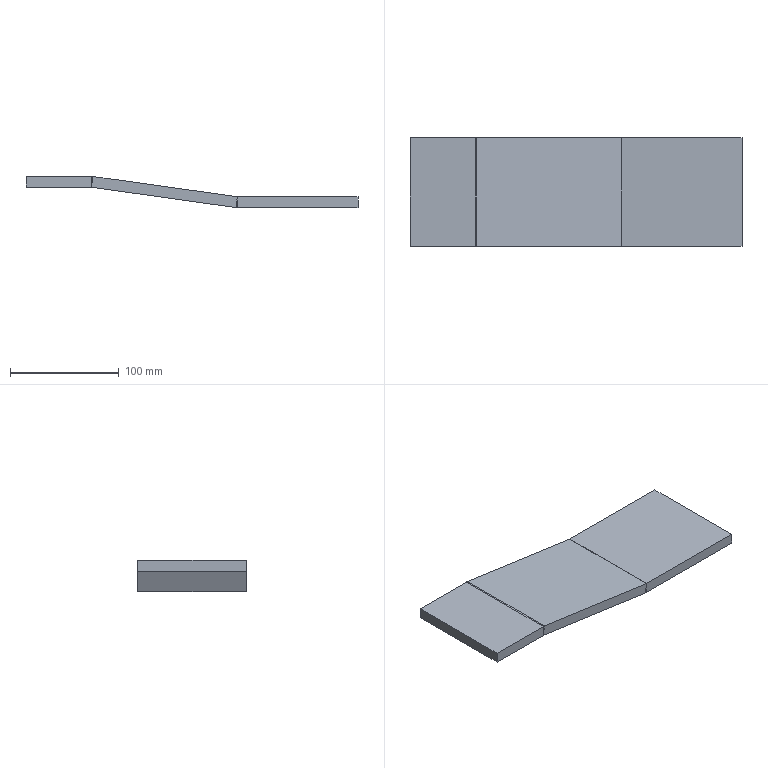Part | STEP file | C1 | 1 solid | 22 faces | box 305.395 x 100 x 28.803 mm | volume 306707 mm3 | plane 18 | cylinder 4 | commonest cylinder face diameters 3 x2 23 x2
STEP:
#1=CARTESIAN_POINT('',(0.,0.,0.));
#2=DIRECTION('',(0.,0.,1.));
#3=DIRECTION('',(1.,0.,0.));
#4=AXIS2_PLACEMENT_3D('',#1,#2,#3);
#5=CARTESIAN_POINT('',(0.,100.,0.));
#6=VERTEX_POINT('',#5);
#7=CARTESIAN_POINT('',(0.,0.,0.));
#8=VERTEX_POINT('',#7);
#9=CARTESIAN_POINT('',(0.,100.,0.));
#10=DIRECTION('',(0.,-1.,0.));
#11=VECTOR('',#10,1.);
#12=LINE('',#9,#11);
#13=CARTESIAN_POINT('',(0.,100.,-10.));
#14=DIRECTION('',(-1.,0.,0.));
#15=DIRECTION('',(0.,-1.,0.));
#16=AXIS2_PLACEMENT_3D('',#13,#14,#15);
#17=PLANE('',#16);
#18=CARTESIAN_POINT('',(0.,10.));
#19=DIRECTION('',(1.,0.));
#20=VECTOR('',#19,1.);
#21=LINE('',#18,#20);
#22=(GEOMETRIC_REPRESENTATION_CONTEXT(2)PARAMETRIC_REPRESENTATION_CONTEXT()REPRESENTATION_CONTEXT('',''));
#23=DEFINITIONAL_REPRESENTATION('',(#21),#22);
#24=PCURVE('',#17,#23);
#25=CARTESIAN_POINT('',(0.,0.,0.));
#26=DIRECTION('',(0.,0.,1.));
#27=DIRECTION('',(1.,0.,0.));
#28=AXIS2_PLACEMENT_3D('',#25,#26,#27);
#29=PLANE('',#28);
#30=CARTESIAN_POINT('',(0.,100.));
#31=DIRECTION('',(0.,-1.));
#32=VECTOR('',#31,1.);
#33=LINE('',#30,#32);
#34=(GEOMETRIC_REPRESENTATION_CONTEXT(2)PARAMETRIC_REPRESENTATION_CONTEXT()REPRESENTATION_CONTEXT('',''));
#35=DEFINITIONAL_REPRESENTATION('',(#33),#34);
#36=PCURVE('',#29,#35);
#37=SURFACE_CURVE('',#12,(#24,#36),.PCURVE_S1.);
#38=EDGE_CURVE('',#6,#8,#37,.T.);
#39=ORIENTED_EDGE('',*,*,#38,.F.);
#40=CARTESIAN_POINT('',(0.,100.,-10.));
#41=VERTEX_POINT('',#40);
#42=CARTESIAN_POINT('',(0.,100.,-10.));
#43=DIRECTION('',(0.,0.,1.));
#44=VECTOR('',#43,1.);
#45=LINE('',#42,#44);
#46=CARTESIAN_POINT('',(0.,0.));
#47=DIRECTION('',(0.,1.));
#48=VECTOR('',#47,1.);
#49=LINE('',#46,#48);
#50=(GEOMETRIC_REPRESENTATION_CONTEXT(2)PARAMETRIC_REPRESENTATION_CONTEXT()REPRESENTATION_CONTEXT('',''));
#51=DEFINITIONAL_REPRESENTATION('',(#49),#50);
#52=PCURVE('',#17,#51);
#53=CARTESIAN_POINT('',(0.,100.,-10.));
#54=DIRECTION('',(0.,1.,0.));
#55=DIRECTION('',(-1.,0.,0.));
#56=AXIS2_PLACEMENT_3D('',#53,#54,#55);
#57=PLANE('',#56);
#58=CARTESIAN_POINT('',(0.,0.));
#59=DIRECTION('',(0.,1.));
#60=VECTOR('',#59,1.);
#61=LINE('',#58,#60);
#62=(GEOMETRIC_REPRESENTATION_CONTEXT(2)PARAMETRIC_REPRESENTATION_CONTEXT()REPRESENTATION_CONTEXT('',''));
#63=DEFINITIONAL_REPRESENTATION('',(#61),#62);
#64=PCURVE('',#57,#63);
#65=SURFACE_CURVE('',#45,(#52,#64),.PCURVE_S1.);
#66=EDGE_CURVE('',#41,#6,#65,.T.);
#67=ORIENTED_EDGE('',*,*,#66,.F.);
#68=CARTESIAN_POINT('',(0.,0.,-10.));
#69=VERTEX_POINT('',#68);
#70=CARTESIAN_POINT('',(0.,100.,-10.));
#71=DIRECTION('',(0.,-1.,0.));
#72=VECTOR('',#71,1.);
#73=LINE('',#70,#72);
#74=CARTESIAN_POINT('',(0.,0.));
#75=DIRECTION('',(1.,0.));
#76=VECTOR('',#75,1.);
#77=LINE('',#74,#76);
#78=(GEOMETRIC_REPRESENTATION_CONTEXT(2)PARAMETRIC_REPRESENTATION_CONTEXT()REPRESENTATION_CONTEXT('',''));
#79=DEFINITIONAL_REPRESENTATION('',(#77),#78);
#80=PCURVE('',#17,#79);
#81=CARTESIAN_POINT('',(0.,0.,-10.));
#82=DIRECTION('',(0.,0.,1.));
#83=DIRECTION('',(1.,0.,0.));
#84=AXIS2_PLACEMENT_3D('',#81,#82,#83);
#85=PLANE('',#84);
#86=CARTESIAN_POINT('',(0.,100.));
#87=DIRECTION('',(0.,-1.));
#88=VECTOR('',#87,1.);
#89=LINE('',#86,#88);
#90=(GEOMETRIC_REPRESENTATION_CONTEXT(2)PARAMETRIC_REPRESENTATION_CONTEXT()REPRESENTATION_CONTEXT('',''));
#91=DEFINITIONAL_REPRESENTATION('',(#89),#90);
#92=PCURVE('',#85,#91);
#93=SURFACE_CURVE('',#73,(#80,#92),.PCURVE_S1.);
#94=EDGE_CURVE('',#41,#69,#93,.T.);
#95=ORIENTED_EDGE('',*,*,#94,.T.);
#96=CARTESIAN_POINT('',(0.,0.,-10.));
#97=DIRECTION('',(0.,0.,1.));
#98=VECTOR('',#97,1.);
#99=LINE('',#96,#98);
#100=CARTESIAN_POINT('',(100.,0.));
#101=DIRECTION('',(0.,1.));
#102=VECTOR('',#101,1.);
#103=LINE('',#100,#102);
#104=(GEOMETRIC_REPRESENTATION_CONTEXT(2)PARAMETRIC_REPRESENTATION_CONTEXT()REPRESENTATION_CONTEXT('',''));
#105=DEFINITIONAL_REPRESENTATION('',(#103),#104);
#106=PCURVE('',#17,#105);
#107=CARTESIAN_POINT('',(0.,0.,-10.));
#108=DIRECTION('',(0.,-1.,0.));
#109=DIRECTION('',(1.,0.,0.));
#110=AXIS2_PLACEMENT_3D('',#107,#108,#109);
#111=PLANE('',#110);
#112=CARTESIAN_POINT('',(0.,0.));
#113=DIRECTION('',(0.,1.));
#114=VECTOR('',#113,1.);
#115=LINE('',#112,#114);
#116=(GEOMETRIC_REPRESENTATION_CONTEXT(2)PARAMETRIC_REPRESENTATION_CONTEXT()REPRESENTATION_CONTEXT('',''));
#117=DEFINITIONAL_REPRESENTATION('',(#115),#116);
#118=PCURVE('',#111,#117);
#119=SURFACE_CURVE('',#99,(#106,#118),.PCURVE_S1.);
#120=EDGE_CURVE('',#69,#8,#119,.T.);
#121=ORIENTED_EDGE('',*,*,#120,.T.);
#122=EDGE_LOOP('',(#39,#67,#95,#121));
#123=FACE_BOUND('',#122,.T.);
#124=ADVANCED_FACE('',(#123),#17,.T.);
#125=CARTESIAN_POINT('',(60.,100.,0.));
#126=VERTEX_POINT('',#125);
#127=CARTESIAN_POINT('',(0.,100.,0.));
#128=DIRECTION('',(-1.,0.,0.));
#129=VECTOR('',#128,1.);
#130=LINE('',#127,#129);
#131=CARTESIAN_POINT('',(0.,10.));
#132=DIRECTION('',(1.,0.));
#133=VECTOR('',#132,1.);
#134=LINE('',#131,#133);
#135=(GEOMETRIC_REPRESENTATION_CONTEXT(2)PARAMETRIC_REPRESENTATION_CONTEXT()REPRESENTATION_CONTEXT('',''));
#136=DEFINITIONAL_REPRESENTATION('',(#134),#135);
#137=PCURVE('',#57,#136);
#138=CARTESIAN_POINT('',(0.,100.));
#139=DIRECTION('',(-1.,0.));
#140=VECTOR('',#139,1.);
#141=LINE('',#138,#140);
#142=(GEOMETRIC_REPRESENTATION_CONTEXT(2)PARAMETRIC_REPRESENTATION_CONTEXT()REPRESENTATION_CONTEXT('',''));
#143=DEFINITIONAL_REPRESENTATION('',(#141),#142);
#144=PCURVE('',#29,#143);
#145=SURFACE_CURVE('',#130,(#137,#144),.PCURVE_S1.);
#146=EDGE_CURVE('',#126,#6,#145,.T.);
#147=ORIENTED_EDGE('',*,*,#146,.F.);
#148=CARTESIAN_POINT('',(60.,100.,-10.));
#149=VERTEX_POINT('',#148);
#150=CARTESIAN_POINT('',(60.,100.,-10.));
#151=DIRECTION('',(0.,0.,1.));
#152=VECTOR('',#151,1.);
#153=LINE('',#150,#152);
#154=CARTESIAN_POINT('',(-60.,0.));
#155=DIRECTION('',(0.,1.));
#156=VECTOR('',#155,1.);
#157=LINE('',#154,#156);
#158=(GEOMETRIC_REPRESENTATION_CONTEXT(2)PARAMETRIC_REPRESENTATION_CONTEXT()REPRESENTATION_CONTEXT('',''));
#159=DEFINITIONAL_REPRESENTATION('',(#157),#158);
#160=PCURVE('',#57,#159);
#161=CARTESIAN_POINT('',(60.,100.,-11.5));
#162=DIRECTION('',(0.,1.,0.));
#163=DIRECTION('',(0.,0.,1.));
#164=AXIS2_PLACEMENT_3D('',#161,#162,#163);
#165=PLANE('',#164);
#166=CARTESIAN_POINT('',(1.5,0.));
#167=DIRECTION('',(1.,0.));
#168=VECTOR('',#167,1.);
#169=LINE('',#166,#168);
#170=(GEOMETRIC_REPRESENTATION_CONTEXT(2)PARAMETRIC_REPRESENTATION_CONTEXT()REPRESENTATION_CONTEXT('',''));
#171=DEFINITIONAL_REPRESENTATION('',(#169),#170);
#172=PCURVE('',#165,#171);
#173=SURFACE_CURVE('',#153,(#160,#172),.PCURVE_S1.);
#174=EDGE_CURVE('',#149,#126,#173,.T.);
#175=ORIENTED_EDGE('',*,*,#174,.F.);
#176=CARTESIAN_POINT('',(0.,100.,-10.));
#177=DIRECTION('',(-1.,0.,0.));
#178=VECTOR('',#177,1.);
#179=LINE('',#176,#178);
#180=CARTESIAN_POINT('',(0.,0.));
#181=DIRECTION('',(1.,0.));
#182=VECTOR('',#181,1.);
#183=LINE('',#180,#182);
#184=(GEOMETRIC_REPRESENTATION_CONTEXT(2)PARAMETRIC_REPRESENTATION_CONTEXT()REPRESENTATION_CONTEXT('',''));
#185=DEFINITIONAL_REPRESENTATION('',(#183),#184);
#186=PCURVE('',#57,#185);
#187=CARTESIAN_POINT('',(0.,100.));
#188=DIRECTION('',(-1.,0.));
#189=VECTOR('',#188,1.);
#190=LINE('',#187,#189);
#191=(GEOMETRIC_REPRESENTATION_CONTEXT(2)PARAMETRIC_REPRESENTATION_CONTEXT()REPRESENTATION_CONTEXT('',''));
#192=DEFINITIONAL_REPRESENTATION('',(#190),#191);
#193=PCURVE('',#85,#192);
#194=SURFACE_CURVE('',#179,(#186,#193),.PCURVE_S1.);
#195=EDGE_CURVE('',#149,#41,#194,.T.);
#196=ORIENTED_EDGE('',*,*,#195,.T.);
#197=ORIENTED_EDGE('',*,*,#66,.T.);
#198=EDGE_LOOP('',(#147,#175,#196,#197));
#199=FACE_BOUND('',#198,.T.);
#200=ADVANCED_FACE('',(#199),#57,.T.);
#201=CARTESIAN_POINT('',(60.,0.,0.));
#202=VERTEX_POINT('',#201);
#203=CARTESIAN_POINT('',(0.,0.,0.));
#204=DIRECTION('',(1.,0.,0.));
#205=VECTOR('',#204,1.);
#206=LINE('',#203,#205);
#207=CARTESIAN_POINT('',(0.,10.));
#208=DIRECTION('',(1.,0.));
#209=VECTOR('',#208,1.);
#210=LINE('',#207,#209);
#211=(GEOMETRIC_REPRESENTATION_CONTEXT(2)PARAMETRIC_REPRESENTATION_CONTEXT()REPRESENTATION_CONTEXT('',''));
#212=DEFINITIONAL_REPRESENTATION('',(#210),#211);
#213=PCURVE('',#111,#212);
#214=CARTESIAN_POINT('',(0.,0.));
#215=DIRECTION('',(1.,0.));
#216=VECTOR('',#215,1.);
#217=LINE('',#214,#216);
#218=(GEOMETRIC_REPRESENTATION_CONTEXT(2)PARAMETRIC_REPRESENTATION_CONTEXT()REPRESENTATION_CONTEXT('',''));
#219=DEFINITIONAL_REPRESENTATION('',(#217),#218);
#220=PCURVE('',#29,#219);
#221=SURFACE_CURVE('',#206,(#213,#220),.PCURVE_S1.);
#222=EDGE_CURVE('',#8,#202,#221,.T.);
#223=ORIENTED_EDGE('',*,*,#222,.F.);
#224=ORIENTED_EDGE('',*,*,#120,.F.);
#225=CARTESIAN_POINT('',(60.,0.,-10.));
#226=VERTEX_POINT('',#225);
#227=CARTESIAN_POINT('',(0.,0.,-10.));
#228=DIRECTION('',(1.,0.,0.));
#229=VECTOR('',#228,1.);
#230=LINE('',#227,#229);
#231=CARTESIAN_POINT('',(0.,0.));
#232=DIRECTION('',(1.,0.));
#233=VECTOR('',#232,1.);
#234=LINE('',#231,#233);
#235=(GEOMETRIC_REPRESENTATION_CONTEXT(2)PARAMETRIC_REPRESENTATION_CONTEXT()REPRESENTATION_CONTEXT('',''));
#236=DEFINITIONAL_REPRESENTATION('',(#234),#235);
#237=PCURVE('',#111,#236);
#238=CARTESIAN_POINT('',(0.,0.));
#239=DIRECTION('',(1.,0.));
#240=VECTOR('',#239,1.);
#241=LINE('',#238,#240);
#242=(GEOMETRIC_REPRESENTATION_CONTEXT(2)PARAMETRIC_REPRESENTATION_CONTEXT()REPRESENTATION_CONTEXT('',''));
#243=DEFINITIONAL_REPRESENTATION('',(#241),#242);
#244=PCURVE('',#85,#243);
#245=SURFACE_CURVE('',#230,(#237,#244),.PCURVE_S1.);
#246=EDGE_CURVE('',#69,#226,#245,.T.);
#247=ORIENTED_EDGE('',*,*,#246,.T.);
#248=CARTESIAN_POINT('',(60.,0.,-10.));
#249=DIRECTION('',(0.,0.,1.));
#250=VECTOR('',#249,1.);
#251=LINE('',#248,#250);
#252=CARTESIAN_POINT('',(60.,0.));
#253=DIRECTION('',(0.,1.));
#254=VECTOR('',#253,1.);
#255=LINE('',#252,#254);
#256=(GEOMETRIC_REPRESENTATION_CONTEXT(2)PARAMETRIC_REPRESENTATION_CONTEXT()REPRESENTATION_CONTEXT('',''));
#257=DEFINITIONAL_REPRESENTATION('',(#255),#256);
#258=PCURVE('',#111,#257);
#259=CARTESIAN_POINT('',(60.,0.,-11.5));
#260=DIRECTION('',(0.,1.,0.));
#261=DIRECTION('',(0.,0.,1.));
#262=AXIS2_PLACEMENT_3D('',#259,#260,#261);
#263=PLANE('',#262);
#264=CARTESIAN_POINT('',(1.5,0.));
#265=DIRECTION('',(1.,0.));
#266=VECTOR('',#265,1.);
#267=LINE('',#264,#266);
#268=(GEOMETRIC_REPRESENTATION_CONTEXT(2)PARAMETRIC_REPRESENTATION_CONTEXT()REPRESENTATION_CONTEXT('',''));
#269=DEFINITIONAL_REPRESENTATION('',(#267),#268);
#270=PCURVE('',#263,#269);
#271=SURFACE_CURVE('',#251,(#258,#270),.PCURVE_S1.);
#272=EDGE_CURVE('',#226,#202,#271,.T.);
#273=ORIENTED_EDGE('',*,*,#272,.T.);
#274=EDGE_LOOP('',(#223,#224,#247,#273));
#275=FACE_BOUND('',#274,.T.);
#276=ADVANCED_FACE('',(#275),#111,.T.);
#277=ORIENTED_EDGE('',*,*,#94,.F.);
#278=ORIENTED_EDGE('',*,*,#195,.F.);
#279=CARTESIAN_POINT('',(60.,100.,-10.));
#280=DIRECTION('',(0.,1.,0.));
#281=VECTOR('',#280,1.);
#282=LINE('',#279,#281);
#283=CARTESIAN_POINT('',(60.,100.));
#284=DIRECTION('',(0.,1.));
#285=VECTOR('',#284,1.);
#286=LINE('',#283,#285);
#287=(GEOMETRIC_REPRESENTATION_CONTEXT(2)PARAMETRIC_REPRESENTATION_CONTEXT()REPRESENTATION_CONTEXT('',''));
#288=DEFINITIONAL_REPRESENTATION('',(#286),#287);
#289=PCURVE('',#85,#288);
#290=CARTESIAN_POINT('',(60.,0.,-11.5));
#291=DIRECTION('',(0.,-1.,0.));
#292=DIRECTION('',(0.1392,0.,0.9903));
#293=AXIS2_PLACEMENT_3D('',#290,#291,#292);
#294=CYLINDRICAL_SURFACE('',#293,1.5);
#295=CARTESIAN_POINT('',(0.1396,-100.));
#296=DIRECTION('',(0.,-1.));
#297=VECTOR('',#296,1.);
#298=LINE('',#295,#297);
#299=(GEOMETRIC_REPRESENTATION_CONTEXT(2)PARAMETRIC_REPRESENTATION_CONTEXT()REPRESENTATION_CONTEXT('',''));
#300=DEFINITIONAL_REPRESENTATION('',(#298),#299);
#301=PCURVE('',#294,#300);
#302=SURFACE_CURVE('',#282,(#289,#301),.PCURVE_S1.);
#303=EDGE_CURVE('',#226,#149,#302,.T.);
#304=ORIENTED_EDGE('',*,*,#303,.F.);
#305=ORIENTED_EDGE('',*,*,#246,.F.);
#306=EDGE_LOOP('',(#277,#278,#304,#305));
#307=FACE_BOUND('',#306,.T.);
#308=ADVANCED_FACE('',(#307),#85,.F.);
#309=ORIENTED_EDGE('',*,*,#38,.T.);
#310=ORIENTED_EDGE('',*,*,#222,.T.);
#311=CARTESIAN_POINT('',(60.,100.,0.));
#312=DIRECTION('',(0.,1.,0.));
#313=VECTOR('',#312,1.);
#314=LINE('',#311,#313);
#315=CARTESIAN_POINT('',(60.,100.));
#316=DIRECTION('',(0.,1.));
#317=VECTOR('',#316,1.);
#318=LINE('',#315,#317);
#319=(GEOMETRIC_REPRESENTATION_CONTEXT(2)PARAMETRIC_REPRESENTATION_CONTEXT()REPRESENTATION_CONTEXT('',''));
#320=DEFINITIONAL_REPRESENTATION('',(#318),#319);
#321=PCURVE('',#29,#320);
#322=CARTESIAN_POINT('',(60.,0.,-11.5));
#323=DIRECTION('',(0.,-1.,0.));
#324=DIRECTION('',(0.1392,0.,0.9903));
#325=AXIS2_PLACEMENT_3D('',#322,#323,#324);
#326=CYLINDRICAL_SURFACE('',#325,11.5);
#327=CARTESIAN_POINT('',(0.1396,-100.));
#328=DIRECTION('',(0.,-1.));
#329=VECTOR('',#328,1.);
#330=LINE('',#327,#329);
#331=(GEOMETRIC_REPRESENTATION_CONTEXT(2)PARAMETRIC_REPRESENTATION_CONTEXT()REPRESENTATION_CONTEXT('',''));
#332=DEFINITIONAL_REPRESENTATION('',(#330),#331);
#333=PCURVE('',#326,#332);
#334=SURFACE_CURVE('',#314,(#321,#333),.PCURVE_S1.);
#335=EDGE_CURVE('',#202,#126,#334,.T.);
#336=ORIENTED_EDGE('',*,*,#335,.T.);
#337=ORIENTED_EDGE('',*,*,#146,.T.);
#338=EDGE_LOOP('',(#309,#310,#336,#337));
#339=FACE_BOUND('',#338,.T.);
#340=ADVANCED_FACE('',(#339),#29,.T.);
#341=CARTESIAN_POINT('',(60.209,100.,-10.015));
#342=VERTEX_POINT('',#341);
#343=CARTESIAN_POINT('',(61.6,100.,-0.1119));
#344=VERTEX_POINT('',#343);
#345=CARTESIAN_POINT('',(61.6,100.,-0.1119));
#346=DIRECTION('',(0.1392,0.,0.9903));
#347=VECTOR('',#346,1.);
#348=LINE('',#345,#347);
#349=CARTESIAN_POINT('',(11.388,1.6));
#350=DIRECTION('',(0.9903,0.1392));
#351=VECTOR('',#350,1.);
#352=LINE('',#349,#351);
#353=(GEOMETRIC_REPRESENTATION_CONTEXT(2)PARAMETRIC_REPRESENTATION_CONTEXT()REPRESENTATION_CONTEXT('',''));
#354=DEFINITIONAL_REPRESENTATION('',(#352),#353);
#355=PCURVE('',#165,#354);
#356=CARTESIAN_POINT('',(194.49,100.,-18.788));
#357=DIRECTION('',(0.,1.,0.));
#358=DIRECTION('',(-1.,0.,0.));
#359=AXIS2_PLACEMENT_3D('',#356,#357,#358);
#360=PLANE('',#359);
#361=CARTESIAN_POINT('',(132.89,18.676));
#362=DIRECTION('',(-0.1392,0.9903));
#363=VECTOR('',#362,1.);
#364=LINE('',#361,#363);
#365=(GEOMETRIC_REPRESENTATION_CONTEXT(2)PARAMETRIC_REPRESENTATION_CONTEXT()REPRESENTATION_CONTEXT('',''));
#366=DEFINITIONAL_REPRESENTATION('',(#364),#365);
#367=PCURVE('',#360,#366);
#368=SURFACE_CURVE('',#348,(#355,#367),.PCURVE_S1.);
#369=EDGE_CURVE('',#342,#344,#368,.T.);
#370=ORIENTED_EDGE('',*,*,#369,.F.);
#371=CARTESIAN_POINT('',(60.,100.,-11.5));
#372=DIRECTION('',(0.,1.,0.));
#373=DIRECTION('',(0.,0.,-1.));
#374=AXIS2_PLACEMENT_3D('',#371,#372,#373);
#375=CIRCLE('',#374,1.5);
#376=CARTESIAN_POINT('',(0.,0.));
#377=DIRECTION('',(-1.,0.));
#378=AXIS2_PLACEMENT_2D('',#376,#377);
#379=CIRCLE('',#378,1.5);
#380=(GEOMETRIC_REPRESENTATION_CONTEXT(2)PARAMETRIC_REPRESENTATION_CONTEXT()REPRESENTATION_CONTEXT('',''));
#381=DEFINITIONAL_REPRESENTATION('',(#379),#380);
#382=PCURVE('',#165,#381);
#383=CARTESIAN_POINT('',(3.281,-100.));
#384=DIRECTION('',(-1.,0.));
#385=VECTOR('',#384,1.);
#386=LINE('',#383,#385);
#387=(GEOMETRIC_REPRESENTATION_CONTEXT(2)PARAMETRIC_REPRESENTATION_CONTEXT()REPRESENTATION_CONTEXT('',''));
#388=DEFINITIONAL_REPRESENTATION('',(#386),#387);
#389=PCURVE('',#294,#388);
#390=SURFACE_CURVE('',#375,(#382,#389),.PCURVE_S1.);
#391=EDGE_CURVE('',#149,#342,#390,.T.);
#392=ORIENTED_EDGE('',*,*,#391,.F.);
#393=ORIENTED_EDGE('',*,*,#174,.T.);
#394=CARTESIAN_POINT('',(60.,100.,-11.5));
#395=DIRECTION('',(0.,1.,0.));
#396=DIRECTION('',(0.,0.,-1.));
#397=AXIS2_PLACEMENT_3D('',#394,#395,#396);
#398=CIRCLE('',#397,11.5);
#399=CARTESIAN_POINT('',(0.,0.));
#400=DIRECTION('',(-1.,0.));
#401=AXIS2_PLACEMENT_2D('',#399,#400);
#402=CIRCLE('',#401,11.5);
#403=(GEOMETRIC_REPRESENTATION_CONTEXT(2)PARAMETRIC_REPRESENTATION_CONTEXT()REPRESENTATION_CONTEXT('',''));
#404=DEFINITIONAL_REPRESENTATION('',(#402),#403);
#405=PCURVE('',#165,#404);
#406=CARTESIAN_POINT('',(3.281,-100.));
#407=DIRECTION('',(-1.,0.));
#408=VECTOR('',#407,1.);
#409=LINE('',#406,#408);
#410=(GEOMETRIC_REPRESENTATION_CONTEXT(2)PARAMETRIC_REPRESENTATION_CONTEXT()REPRESENTATION_CONTEXT('',''));
#411=DEFINITIONAL_REPRESENTATION('',(#409),#410);
#412=PCURVE('',#326,#411);
#413=SURFACE_CURVE('',#398,(#405,#412),.PCURVE_S1.);
#414=EDGE_CURVE('',#126,#344,#413,.T.);
#415=ORIENTED_EDGE('',*,*,#414,.T.);
#416=EDGE_LOOP('',(#370,#392,#393,#415));
#417=FACE_BOUND('',#416,.T.);
#418=ADVANCED_FACE('',(#417),#165,.T.);
#419=CARTESIAN_POINT('',(60.209,0.,-10.015));
#420=VERTEX_POINT('',#419);
#421=CARTESIAN_POINT('',(60.,0.,-11.5));
#422=DIRECTION('',(0.,-1.,0.));
#423=DIRECTION('',(0.,0.,-1.));
#424=AXIS2_PLACEMENT_3D('',#421,#422,#423);
#425=CIRCLE('',#424,1.5);
#426=CARTESIAN_POINT('',(-1.5,0.));
#427=CARTESIAN_POINT('',(-1.5,2.598));
#428=CARTESIAN_POINT('',(0.75,1.299));
#429=CARTESIAN_POINT('',(3.,0.));
#430=CARTESIAN_POINT('',(0.75,-1.299));
#431=CARTESIAN_POINT('',(-1.5,-2.598));
#432=CARTESIAN_POINT('',(-1.5,0.));
#433=(BOUNDED_CURVE()B_SPLINE_CURVE(2,(#426,#427,#428,#429,#430,#431,#432),.UNSPECIFIED.,.T.,.F.)B_SPLINE_CURVE_WITH_KNOTS((1,2,2,2,2,1),(-2.094,0.,2.094,4.189,6.283,8.378),.UNSPECIFIED.)CURVE()GEOMETRIC_REPRESENTATION_ITEM()RATIONAL_B_SPLINE_CURVE((1.,0.5,1.,0.5,1.,0.5,1.))REPRESENTATION_ITEM(''));
#434=(GEOMETRIC_REPRESENTATION_CONTEXT(2)PARAMETRIC_REPRESENTATION_CONTEXT()REPRESENTATION_CONTEXT('',''));
#435=DEFINITIONAL_REPRESENTATION('',(#433),#434);
#436=PCURVE('',#263,#435);
#437=CARTESIAN_POINT('',(-3.002,0.));
#438=DIRECTION('',(1.,0.));
#439=VECTOR('',#438,1.);
#440=LINE('',#437,#439);
#441=(GEOMETRIC_REPRESENTATION_CONTEXT(2)PARAMETRIC_REPRESENTATION_CONTEXT()REPRESENTATION_CONTEXT('',''));
#442=DEFINITIONAL_REPRESENTATION('',(#440),#441);
#443=PCURVE('',#294,#442);
#444=SURFACE_CURVE('',#425,(#436,#443),.PCURVE_S1.);
#445=EDGE_CURVE('',#420,#226,#444,.T.);
#446=ORIENTED_EDGE('',*,*,#445,.F.);
#447=CARTESIAN_POINT('',(61.6,0.,-0.1119));
#448=VERTEX_POINT('',#447);
#449=CARTESIAN_POINT('',(60.209,0.,-10.015));
#450=DIRECTION('',(0.1392,0.,0.9903));
#451=VECTOR('',#450,1.);
#452=LINE('',#449,#451);
#453=CARTESIAN_POINT('',(1.485,0.2088));
#454=DIRECTION('',(0.9903,0.1392));
#455=VECTOR('',#454,1.);
#456=LINE('',#453,#455);
#457=(GEOMETRIC_REPRESENTATION_CONTEXT(2)PARAMETRIC_REPRESENTATION_CONTEXT()REPRESENTATION_CONTEXT('',''));
#458=DEFINITIONAL_REPRESENTATION('',(#456),#457);
#459=PCURVE('',#263,#458);
#460=CARTESIAN_POINT('',(61.497,0.,-0.09732));
#461=DIRECTION('',(0.,-1.,0.));
#462=DIRECTION('',(1.,0.,0.));
#463=AXIS2_PLACEMENT_3D('',#460,#461,#462);
#464=PLANE('',#463);
#465=CARTESIAN_POINT('',(-1.288,-9.917));
#466=DIRECTION('',(0.1392,0.9903));
#467=VECTOR('',#466,1.);
#468=LINE('',#465,#467);
#469=(GEOMETRIC_REPRESENTATION_CONTEXT(2)PARAMETRIC_REPRESENTATION_CONTEXT()REPRESENTATION_CONTEXT('',''));
#470=DEFINITIONAL_REPRESENTATION('',(#468),#469);
#471=PCURVE('',#464,#470);
#472=SURFACE_CURVE('',#452,(#459,#471),.PCURVE_S1.);
#473=EDGE_CURVE('',#420,#448,#472,.T.);
#474=ORIENTED_EDGE('',*,*,#473,.T.);
#475=CARTESIAN_POINT('',(60.,0.,-11.5));
#476=DIRECTION('',(0.,-1.,0.));
#477=DIRECTION('',(0.,0.,-1.));
#478=AXIS2_PLACEMENT_3D('',#475,#476,#477);
#479=CIRCLE('',#478,11.5);
#480=CARTESIAN_POINT('',(-11.5,0.));
#481=CARTESIAN_POINT('',(-11.5,19.919));
#482=CARTESIAN_POINT('',(5.75,9.959));
#483=CARTESIAN_POINT('',(23.,0.));
#484=CARTESIAN_POINT('',(5.75,-9.959));
#485=CARTESIAN_POINT('',(-11.5,-19.919));
#486=CARTESIAN_POINT('',(-11.5,0.));
#487=(BOUNDED_CURVE()B_SPLINE_CURVE(2,(#480,#481,#482,#483,#484,#485,#486),.UNSPECIFIED.,.T.,.F.)B_SPLINE_CURVE_WITH_KNOTS((1,2,2,2,2,1),(-2.094,0.,2.094,4.189,6.283,8.378),.UNSPECIFIED.)CURVE()GEOMETRIC_REPRESENTATION_ITEM()RATIONAL_B_SPLINE_CURVE((1.,0.5,1.,0.5,1.,0.5,1.))REPRESENTATION_ITEM(''));
#488=(GEOMETRIC_REPRESENTATION_CONTEXT(2)PARAMETRIC_REPRESENTATION_CONTEXT()REPRESENTATION_CONTEXT('',''));
#489=DEFINITIONAL_REPRESENTATION('',(#487),#488);
#490=PCURVE('',#263,#489);
#491=CARTESIAN_POINT('',(-3.002,0.));
#492=DIRECTION('',(1.,0.));
#493=VECTOR('',#492,1.);
#494=LINE('',#491,#493);
#495=(GEOMETRIC_REPRESENTATION_CONTEXT(2)PARAMETRIC_REPRESENTATION_CONTEXT()REPRESENTATION_CONTEXT('',''));
#496=DEFINITIONAL_REPRESENTATION('',(#494),#495);
#497=PCURVE('',#326,#496);
#498=SURFACE_CURVE('',#479,(#490,#497),.PCURVE_S1.);
#499=EDGE_CURVE('',#448,#202,#498,.T.);
#500=ORIENTED_EDGE('',*,*,#499,.T.);
#501=ORIENTED_EDGE('',*,*,#272,.F.);
#502=EDGE_LOOP('',(#446,#474,#500,#501));
#503=FACE_BOUND('',#502,.T.);
#504=ADVANCED_FACE('',(#503),#263,.F.);
#505=ORIENTED_EDGE('',*,*,#335,.F.);
#506=ORIENTED_EDGE('',*,*,#499,.F.);
#507=CARTESIAN_POINT('',(61.6,0.,-0.1119));
#508=DIRECTION('',(0.,-1.,0.));
#509=VECTOR('',#508,1.);
#510=LINE('',#507,#509);
#511=CARTESIAN_POINT('',(0.,0.));
#512=DIRECTION('',(0.,1.));
#513=VECTOR('',#512,1.);
#514=LINE('',#511,#513);
#515=(GEOMETRIC_REPRESENTATION_CONTEXT(2)PARAMETRIC_REPRESENTATION_CONTEXT()REPRESENTATION_CONTEXT('',''));
#516=DEFINITIONAL_REPRESENTATION('',(#514),#515);
#517=PCURVE('',#326,#516);
#518=CARTESIAN_POINT('',(1.281,0.,8.365));
#519=DIRECTION('',(0.1392,0.,0.9903));
#520=DIRECTION('',(0.9903,0.,-0.1392));
#521=AXIS2_PLACEMENT_3D('',#518,#519,#520);
#522=PLANE('',#521);
#523=CARTESIAN_POINT('',(60.913,0.));
#524=DIRECTION('',(0.,-1.));
#525=VECTOR('',#524,1.);
#526=LINE('',#523,#525);
#527=(GEOMETRIC_REPRESENTATION_CONTEXT(2)PARAMETRIC_REPRESENTATION_CONTEXT()REPRESENTATION_CONTEXT('',''));
#528=DEFINITIONAL_REPRESENTATION('',(#526),#527);
#529=PCURVE('',#522,#528);
#530=SURFACE_CURVE('',#510,(#517,#529),.PCURVE_S1.);
#531=EDGE_CURVE('',#344,#448,#530,.T.);
#532=ORIENTED_EDGE('',*,*,#531,.F.);
#533=ORIENTED_EDGE('',*,*,#414,.F.);
#534=EDGE_LOOP('',(#505,#506,#532,#533));
#535=FACE_BOUND('',#534,.T.);
#536=ADVANCED_FACE('',(#535),#326,.T.);
#537=ORIENTED_EDGE('',*,*,#445,.F.);
#538=CARTESIAN_POINT('',(60.209,100.,-10.015));
#539=DIRECTION('',(0.,-1.,0.));
#540=VECTOR('',#539,1.);
#541=LINE('',#538,#540);
#542=CARTESIAN_POINT('',(0.,-100.));
#543=DIRECTION('',(0.,1.));
#544=VECTOR('',#543,1.);
#545=LINE('',#542,#544);
#546=(GEOMETRIC_REPRESENTATION_CONTEXT(2)PARAMETRIC_REPRESENTATION_CONTEXT()REPRESENTATION_CONTEXT('',''));
#547=DEFINITIONAL_REPRESENTATION('',(#545),#546);
#548=PCURVE('',#294,#547);
#549=CARTESIAN_POINT('',(-0.1111,0.,-1.537));
#550=DIRECTION('',(0.1392,0.,0.9903));
#551=DIRECTION('',(0.9903,0.,-0.1392));
#552=AXIS2_PLACEMENT_3D('',#549,#550,#551);
#553=PLANE('',#552);
#554=CARTESIAN_POINT('',(60.913,100.));
#555=DIRECTION('',(0.,-1.));
#556=VECTOR('',#555,1.);
#557=LINE('',#554,#556);
#558=(GEOMETRIC_REPRESENTATION_CONTEXT(2)PARAMETRIC_REPRESENTATION_CONTEXT()REPRESENTATION_CONTEXT('',''));
#559=DEFINITIONAL_REPRESENTATION('',(#557),#558);
#560=PCURVE('',#553,#559);
#561=SURFACE_CURVE('',#541,(#548,#560),.PCURVE_S1.);
#562=EDGE_CURVE('',#342,#420,#561,.T.);
#563=ORIENTED_EDGE('',*,*,#562,.F.);
#564=ORIENTED_EDGE('',*,*,#391,.F.);
#565=ORIENTED_EDGE('',*,*,#303,.F.);
#566=EDGE_LOOP('',(#537,#563,#564,#565));
#567=FACE_BOUND('',#566,.F.);
#568=ADVANCED_FACE('',(#567),#294,.F.);
#569=CARTESIAN_POINT('',(194.49,0.,-18.788));
#570=VERTEX_POINT('',#569);
#571=CARTESIAN_POINT('',(61.497,0.,-0.09732));
#572=DIRECTION('',(-0.9903,0.,0.1392));
#573=VECTOR('',#572,1.);
#574=LINE('',#571,#573);
#575=CARTESIAN_POINT('',(0.,0.));
#576=DIRECTION('',(-0.9903,0.1392));
#577=VECTOR('',#576,1.);
#578=LINE('',#575,#577);
#579=(GEOMETRIC_REPRESENTATION_CONTEXT(2)PARAMETRIC_REPRESENTATION_CONTEXT()REPRESENTATION_CONTEXT('',''));
#580=DEFINITIONAL_REPRESENTATION('',(#578),#579);
#581=PCURVE('',#464,#580);
#582=CARTESIAN_POINT('',(60.808,0.));
#583=DIRECTION('',(-1.,0.));
#584=VECTOR('',#583,1.);
#585=LINE('',#582,#584);
#586=(GEOMETRIC_REPRESENTATION_CONTEXT(2)PARAMETRIC_REPRESENTATION_CONTEXT()REPRESENTATION_CONTEXT('',''));
#587=DEFINITIONAL_REPRESENTATION('',(#585),#586);
#588=PCURVE('',#522,#587);
#589=SURFACE_CURVE('',#574,(#581,#588),.PCURVE_S1.);
#590=EDGE_CURVE('',#570,#448,#589,.T.);
#591=ORIENTED_EDGE('',*,*,#590,.T.);
#592=ORIENTED_EDGE('',*,*,#473,.F.);
#593=CARTESIAN_POINT('',(193.099,0.,-28.691));
#594=VERTEX_POINT('',#593);
#595=CARTESIAN_POINT('',(-0.1111,0.,-1.537));
#596=DIRECTION('',(-0.9903,0.,0.1392));
#597=VECTOR('',#596,1.);
#598=LINE('',#595,#597);
#599=CARTESIAN_POINT('',(-61.608,-1.44));
#600=DIRECTION('',(-0.9903,0.1392));
#601=VECTOR('',#600,1.);
#602=LINE('',#599,#601);
#603=(GEOMETRIC_REPRESENTATION_CONTEXT(2)PARAMETRIC_REPRESENTATION_CONTEXT()REPRESENTATION_CONTEXT('',''));
#604=DEFINITIONAL_REPRESENTATION('',(#602),#603);
#605=PCURVE('',#464,#604);
#606=CARTESIAN_POINT('',(0.,0.));
#607=DIRECTION('',(-1.,0.));
#608=VECTOR('',#607,1.);
#609=LINE('',#606,#608);
#610=(GEOMETRIC_REPRESENTATION_CONTEXT(2)PARAMETRIC_REPRESENTATION_CONTEXT()REPRESENTATION_CONTEXT('',''));
#611=DEFINITIONAL_REPRESENTATION('',(#609),#610);
#612=PCURVE('',#553,#611);
#613=SURFACE_CURVE('',#598,(#605,#612),.PCURVE_S1.);
#614=EDGE_CURVE('',#594,#420,#613,.T.);
#615=ORIENTED_EDGE('',*,*,#614,.F.);
#616=CARTESIAN_POINT('',(194.49,0.,-18.788));
#617=DIRECTION('',(-0.1392,0.,-0.9903));
#618=VECTOR('',#617,1.);
#619=LINE('',#616,#618);
#620=CARTESIAN_POINT('',(132.994,-18.691));
#621=DIRECTION('',(-0.1392,-0.9903));
#622=VECTOR('',#621,1.);
#623=LINE('',#620,#622);
#624=(GEOMETRIC_REPRESENTATION_CONTEXT(2)PARAMETRIC_REPRESENTATION_CONTEXT()REPRESENTATION_CONTEXT('',''));
#625=DEFINITIONAL_REPRESENTATION('',(#623),#624);
#626=PCURVE('',#464,#625);
#627=CARTESIAN_POINT('',(194.699,0.,-17.303));
#628=DIRECTION('',(0.,-1.,0.));
#629=DIRECTION('',(0.,0.,-1.));
#630=AXIS2_PLACEMENT_3D('',#627,#628,#629);
#631=PLANE('',#630);
#632=CARTESIAN_POINT('',(1.485,-0.2088));
#633=DIRECTION('',(0.9903,-0.1392));
#634=VECTOR('',#633,1.);
#635=LINE('',#632,#634);
#636=(GEOMETRIC_REPRESENTATION_CONTEXT(2)PARAMETRIC_REPRESENTATION_CONTEXT()REPRESENTATION_CONTEXT('',''));
#637=DEFINITIONAL_REPRESENTATION('',(#635),#636);
#638=PCURVE('',#631,#637);
#639=SURFACE_CURVE('',#619,(#626,#638),.PCURVE_S1.);
#640=EDGE_CURVE('',#570,#594,#639,.T.);
#641=ORIENTED_EDGE('',*,*,#640,.F.);
#642=EDGE_LOOP('',(#591,#592,#615,#641));
#643=FACE_BOUND('',#642,.T.);
#644=ADVANCED_FACE('',(#643),#464,.T.);
#645=CARTESIAN_POINT('',(193.099,100.,-28.691));
#646=VERTEX_POINT('',#645);
#647=CARTESIAN_POINT('',(-0.1111,100.,-1.537));
#648=DIRECTION('',(0.9903,0.,-0.1392));
#649=VECTOR('',#648,1.);
#650=LINE('',#647,#649);
#651=CARTESIAN_POINT('',(194.601,17.251));
#652=DIRECTION('',(-0.9903,-0.1392));
#653=VECTOR('',#652,1.);
#654=LINE('',#651,#653);
#655=(GEOMETRIC_REPRESENTATION_CONTEXT(2)PARAMETRIC_REPRESENTATION_CONTEXT()REPRESENTATION_CONTEXT('',''));
#656=DEFINITIONAL_REPRESENTATION('',(#654),#655);
#657=PCURVE('',#360,#656);
#658=CARTESIAN_POINT('',(0.,100.));
#659=DIRECTION('',(1.,0.));
#660=VECTOR('',#659,1.);
#661=LINE('',#658,#660);
#662=(GEOMETRIC_REPRESENTATION_CONTEXT(2)PARAMETRIC_REPRESENTATION_CONTEXT()REPRESENTATION_CONTEXT('',''));
#663=DEFINITIONAL_REPRESENTATION('',(#661),#662);
#664=PCURVE('',#553,#663);
#665=SURFACE_CURVE('',#650,(#657,#664),.PCURVE_S1.);
#666=EDGE_CURVE('',#342,#646,#665,.T.);
#667=ORIENTED_EDGE('',*,*,#666,.F.);
#668=ORIENTED_EDGE('',*,*,#369,.T.);
#669=CARTESIAN_POINT('',(194.49,100.,-18.788));
#670=VERTEX_POINT('',#669);
#671=CARTESIAN_POINT('',(194.49,100.,-18.788));
#672=DIRECTION('',(0.9903,0.,-0.1392));
#673=VECTOR('',#672,1.);
#674=LINE('',#671,#673);
#675=CARTESIAN_POINT('',(0.,0.));
#676=DIRECTION('',(-0.9903,-0.1392));
#677=VECTOR('',#676,1.);
#678=LINE('',#675,#677);
#679=(GEOMETRIC_REPRESENTATION_CONTEXT(2)PARAMETRIC_REPRESENTATION_CONTEXT()REPRESENTATION_CONTEXT('',''));
#680=DEFINITIONAL_REPRESENTATION('',(#678),#679);
#681=PCURVE('',#360,#680);
#682=CARTESIAN_POINT('',(195.109,100.));
#683=DIRECTION('',(1.,0.));
#684=VECTOR('',#683,1.);
#685=LINE('',#682,#684);
#686=(GEOMETRIC_REPRESENTATION_CONTEXT(2)PARAMETRIC_REPRESENTATION_CONTEXT()REPRESENTATION_CONTEXT('',''));
#687=DEFINITIONAL_REPRESENTATION('',(#685),#686);
#688=PCURVE('',#522,#687);
#689=SURFACE_CURVE('',#674,(#681,#688),.PCURVE_S1.);
#690=EDGE_CURVE('',#344,#670,#689,.T.);
#691=ORIENTED_EDGE('',*,*,#690,.T.);
#692=CARTESIAN_POINT('',(194.49,100.,-18.788));
#693=DIRECTION('',(-0.1392,0.,-0.9903));
#694=VECTOR('',#693,1.);
#695=LINE('',#692,#694);
#696=CARTESIAN_POINT('',(0.,0.));
#697=DIRECTION('',(0.1392,-0.9903));
#698=VECTOR('',#697,1.);
#699=LINE('',#696,#698);
#700=(GEOMETRIC_REPRESENTATION_CONTEXT(2)PARAMETRIC_REPRESENTATION_CONTEXT()REPRESENTATION_CONTEXT('',''));
#701=DEFINITIONAL_REPRESENTATION('',(#699),#700);
#702=PCURVE('',#360,#701);
#703=CARTESIAN_POINT('',(194.699,100.,-17.303));
#704=DIRECTION('',(0.,-1.,0.));
#705=DIRECTION('',(0.,0.,-1.));
#706=AXIS2_PLACEMENT_3D('',#703,#704,#705);
#707=PLANE('',#706);
#708=CARTESIAN_POINT('',(1.485,-0.2088));
#709=DIRECTION('',(0.9903,-0.1392));
#710=VECTOR('',#709,1.);
#711=LINE('',#708,#710);
#712=(GEOMETRIC_REPRESENTATION_CONTEXT(2)PARAMETRIC_REPRESENTATION_CONTEXT()REPRESENTATION_CONTEXT('',''));
#713=DEFINITIONAL_REPRESENTATION('',(#711),#712);
#714=PCURVE('',#707,#713);
#715=SURFACE_CURVE('',#695,(#702,#714),.PCURVE_S1.);
#716=EDGE_CURVE('',#670,#646,#715,.T.);
#717=ORIENTED_EDGE('',*,*,#716,.T.);
#718=EDGE_LOOP('',(#667,#668,#691,#717));
#719=FACE_BOUND('',#718,.T.);
#720=ADVANCED_FACE('',(#719),#360,.T.);
#721=ORIENTED_EDGE('',*,*,#690,.F.);
#722=ORIENTED_EDGE('',*,*,#531,.T.);
#723=ORIENTED_EDGE('',*,*,#590,.F.);
#724=CARTESIAN_POINT('',(194.49,0.,-18.788));
#725=DIRECTION('',(0.,-1.,0.));
#726=VECTOR('',#725,1.);
#727=LINE('',#724,#726);
#728=CARTESIAN_POINT('',(195.109,0.));
#729=DIRECTION('',(0.,-1.));
#730=VECTOR('',#729,1.);
#731=LINE('',#728,#730);
#732=(GEOMETRIC_REPRESENTATION_CONTEXT(2)PARAMETRIC_REPRESENTATION_CONTEXT()REPRESENTATION_CONTEXT('',''));
#733=DEFINITIONAL_REPRESENTATION('',(#731),#732);
#734=PCURVE('',#522,#733);
#735=CARTESIAN_POINT('',(194.699,100.,-17.303));
#736=DIRECTION('',(0.,1.,0.));
#737=DIRECTION('',(0.,0.,-1.));
#738=AXIS2_PLACEMENT_3D('',#735,#736,#737);
#739=CYLINDRICAL_SURFACE('',#738,1.5);
#740=CARTESIAN_POINT('',(0.1396,-100.));
#741=DIRECTION('',(0.,-1.));
#742=VECTOR('',#741,1.);
#743=LINE('',#740,#742);
#744=(GEOMETRIC_REPRESENTATION_CONTEXT(2)PARAMETRIC_REPRESENTATION_CONTEXT()REPRESENTATION_CONTEXT('',''));
#745=DEFINITIONAL_REPRESENTATION('',(#743),#744);
#746=PCURVE('',#739,#745);
#747=SURFACE_CURVE('',#727,(#734,#746),.PCURVE_S1.);
#748=EDGE_CURVE('',#670,#570,#747,.T.);
#749=ORIENTED_EDGE('',*,*,#748,.F.);
#750=EDGE_LOOP('',(#721,#722,#723,#749));
#751=FACE_BOUND('',#750,.T.);
#752=ADVANCED_FACE('',(#751),#522,.T.);
#753=ORIENTED_EDGE('',*,*,#562,.F.);
#754=ORIENTED_EDGE('',*,*,#666,.T.);
#755=CARTESIAN_POINT('',(193.099,0.,-28.691));
#756=DIRECTION('',(0.,-1.,0.));
#757=VECTOR('',#756,1.);
#758=LINE('',#755,#757);
#759=CARTESIAN_POINT('',(195.109,0.));
#760=DIRECTION('',(0.,-1.));
#761=VECTOR('',#760,1.);
#762=LINE('',#759,#761);
#763=(GEOMETRIC_REPRESENTATION_CONTEXT(2)PARAMETRIC_REPRESENTATION_CONTEXT()REPRESENTATION_CONTEXT('',''));
#764=DEFINITIONAL_REPRESENTATION('',(#762),#763);
#765=PCURVE('',#553,#764);
#766=CARTESIAN_POINT('',(194.699,100.,-17.303));
#767=DIRECTION('',(0.,1.,0.));
#768=DIRECTION('',(0.,0.,-1.));
#769=AXIS2_PLACEMENT_3D('',#766,#767,#768);
#770=CYLINDRICAL_SURFACE('',#769,11.5);
#771=CARTESIAN_POINT('',(0.1396,-100.));
#772=DIRECTION('',(0.,-1.));
#773=VECTOR('',#772,1.);
#774=LINE('',#771,#773);
#775=(GEOMETRIC_REPRESENTATION_CONTEXT(2)PARAMETRIC_REPRESENTATION_CONTEXT()REPRESENTATION_CONTEXT('',''));
#776=DEFINITIONAL_REPRESENTATION('',(#774),#775);
#777=PCURVE('',#770,#776);
#778=SURFACE_CURVE('',#758,(#765,#777),.PCURVE_S1.);
#779=EDGE_CURVE('',#646,#594,#778,.T.);
#780=ORIENTED_EDGE('',*,*,#779,.T.);
#781=ORIENTED_EDGE('',*,*,#614,.T.);
#782=EDGE_LOOP('',(#753,#754,#780,#781));
#783=FACE_BOUND('',#782,.T.);
#784=ADVANCED_FACE('',(#783),#553,.F.);
#785=CARTESIAN_POINT('',(194.699,0.,-18.803));
#786=VERTEX_POINT('',#785);
#787=CARTESIAN_POINT('',(194.699,0.,-28.803));
#788=VERTEX_POINT('',#787);
#789=CARTESIAN_POINT('',(194.699,0.,-28.803));
#790=DIRECTION('',(0.,0.,-1.));
#791=VECTOR('',#790,1.);
#792=LINE('',#789,#791);
#793=CARTESIAN_POINT('',(11.5,0.));
#794=DIRECTION('',(1.,0.));
#795=VECTOR('',#794,1.);
#796=LINE('',#793,#795);
#797=(GEOMETRIC_REPRESENTATION_CONTEXT(2)PARAMETRIC_REPRESENTATION_CONTEXT()REPRESENTATION_CONTEXT('',''));
#798=DEFINITIONAL_REPRESENTATION('',(#796),#797);
#799=PCURVE('',#631,#798);
#800=CARTESIAN_POINT('',(305.395,0.,-28.803));
#801=DIRECTION('',(0.,1.,0.));
#802=DIRECTION('',(-1.,0.,0.));
#803=AXIS2_PLACEMENT_3D('',#800,#801,#802);
#804=PLANE('',#803);
#805=CARTESIAN_POINT('',(110.696,0.));
#806=DIRECTION('',(0.,-1.));
#807=VECTOR('',#806,1.);
#808=LINE('',#805,#807);
#809=(GEOMETRIC_REPRESENTATION_CONTEXT(2)PARAMETRIC_REPRESENTATION_CONTEXT()REPRESENTATION_CONTEXT('',''));
#810=DEFINITIONAL_REPRESENTATION('',(#808),#809);
#811=PCURVE('',#804,#810);
#812=SURFACE_CURVE('',#792,(#799,#811),.PCURVE_S1.);
#813=EDGE_CURVE('',#786,#788,#812,.T.);
#814=ORIENTED_EDGE('',*,*,#813,.F.);
#815=CARTESIAN_POINT('',(194.699,0.,-17.303));
#816=DIRECTION('',(0.,-1.,0.));
#817=DIRECTION('',(0.,0.,1.));
#818=AXIS2_PLACEMENT_3D('',#815,#816,#817);
#819=CIRCLE('',#818,1.5);
#820=CARTESIAN_POINT('',(0.,0.));
#821=DIRECTION('',(-1.,0.));
#822=AXIS2_PLACEMENT_2D('',#820,#821);
#823=CIRCLE('',#822,1.5);
#824=(GEOMETRIC_REPRESENTATION_CONTEXT(2)PARAMETRIC_REPRESENTATION_CONTEXT()REPRESENTATION_CONTEXT('',''));
#825=DEFINITIONAL_REPRESENTATION('',(#823),#824);
#826=PCURVE('',#631,#825);
#827=CARTESIAN_POINT('',(3.142,-100.));
#828=DIRECTION('',(-1.,0.));
#829=VECTOR('',#828,1.);
#830=LINE('',#827,#829);
#831=(GEOMETRIC_REPRESENTATION_CONTEXT(2)PARAMETRIC_REPRESENTATION_CONTEXT()REPRESENTATION_CONTEXT('',''));
#832=DEFINITIONAL_REPRESENTATION('',(#830),#831);
#833=PCURVE('',#739,#832);
#834=SURFACE_CURVE('',#819,(#826,#833),.PCURVE_S1.);
#835=EDGE_CURVE('',#570,#786,#834,.T.);
#836=ORIENTED_EDGE('',*,*,#835,.F.);
#837=ORIENTED_EDGE('',*,*,#640,.T.);
#838=CARTESIAN_POINT('',(194.699,0.,-17.303));
#839=DIRECTION('',(0.,-1.,0.));
#840=DIRECTION('',(0.,0.,1.));
#841=AXIS2_PLACEMENT_3D('',#838,#839,#840);
#842=CIRCLE('',#841,11.5);
#843=CARTESIAN_POINT('',(0.,0.));
#844=DIRECTION('',(-1.,0.));
#845=AXIS2_PLACEMENT_2D('',#843,#844);
#846=CIRCLE('',#845,11.5);
#847=(GEOMETRIC_REPRESENTATION_CONTEXT(2)PARAMETRIC_REPRESENTATION_CONTEXT()REPRESENTATION_CONTEXT('',''));
#848=DEFINITIONAL_REPRESENTATION('',(#846),#847);
#849=PCURVE('',#631,#848);
#850=CARTESIAN_POINT('',(3.142,-100.));
#851=DIRECTION('',(-1.,0.));
#852=VECTOR('',#851,1.);
#853=LINE('',#850,#852);
#854=(GEOMETRIC_REPRESENTATION_CONTEXT(2)PARAMETRIC_REPRESENTATION_CONTEXT()REPRESENTATION_CONTEXT('',''));
#855=DEFINITIONAL_REPRESENTATION('',(#853),#854);
#856=PCURVE('',#770,#855);
#857=SURFACE_CURVE('',#842,(#849,#856),.PCURVE_S1.);
#858=EDGE_CURVE('',#594,#788,#857,.T.);
#859=ORIENTED_EDGE('',*,*,#858,.T.);
#860=EDGE_LOOP('',(#814,#836,#837,#859));
#861=FACE_BOUND('',#860,.T.);
#862=ADVANCED_FACE('',(#861),#631,.T.);
#863=CARTESIAN_POINT('',(194.699,100.,-18.803));
#864=VERTEX_POINT('',#863);
#865=CARTESIAN_POINT('',(194.699,100.,-17.303));
#866=DIRECTION('',(0.,1.,0.));
#867=DIRECTION('',(0.,0.,1.));
#868=AXIS2_PLACEMENT_3D('',#865,#866,#867);
#869=CIRCLE('',#868,1.5);
#870=CARTESIAN_POINT('',(-1.5,0.));
#871=CARTESIAN_POINT('',(-1.5,2.598));
#872=CARTESIAN_POINT('',(0.75,1.299));
#873=CARTESIAN_POINT('',(3.,0.));
#874=CARTESIAN_POINT('',(0.75,-1.299));
#875=CARTESIAN_POINT('',(-1.5,-2.598));
#876=CARTESIAN_POINT('',(-1.5,0.));
#877=(BOUNDED_CURVE()B_SPLINE_CURVE(2,(#870,#871,#872,#873,#874,#875,#876),.UNSPECIFIED.,.T.,.F.)B_SPLINE_CURVE_WITH_KNOTS((1,2,2,2,2,1),(-2.094,0.,2.094,4.189,6.283,8.378),.UNSPECIFIED.)CURVE()GEOMETRIC_REPRESENTATION_ITEM()RATIONAL_B_SPLINE_CURVE((1.,0.5,1.,0.5,1.,0.5,1.))REPRESENTATION_ITEM(''));
#878=(GEOMETRIC_REPRESENTATION_CONTEXT(2)PARAMETRIC_REPRESENTATION_CONTEXT()REPRESENTATION_CONTEXT('',''));
#879=DEFINITIONAL_REPRESENTATION('',(#877),#878);
#880=PCURVE('',#707,#879);
#881=CARTESIAN_POINT('',(-3.142,0.));
#882=DIRECTION('',(1.,0.));
#883=VECTOR('',#882,1.);
#884=LINE('',#881,#883);
#885=(GEOMETRIC_REPRESENTATION_CONTEXT(2)PARAMETRIC_REPRESENTATION_CONTEXT()REPRESENTATION_CONTEXT('',''));
#886=DEFINITIONAL_REPRESENTATION('',(#884),#885);
#887=PCURVE('',#739,#886);
#888=SURFACE_CURVE('',#869,(#880,#887),.PCURVE_S1.);
#889=EDGE_CURVE('',#864,#670,#888,.T.);
#890=ORIENTED_EDGE('',*,*,#889,.F.);
#891=CARTESIAN_POINT('',(194.699,100.,-28.803));
#892=VERTEX_POINT('',#891);
#893=CARTESIAN_POINT('',(194.699,100.,-18.803));
#894=DIRECTION('',(0.,0.,-1.));
#895=VECTOR('',#894,1.);
#896=LINE('',#893,#895);
#897=CARTESIAN_POINT('',(1.5,0.));
#898=DIRECTION('',(1.,0.));
#899=VECTOR('',#898,1.);
#900=LINE('',#897,#899);
#901=(GEOMETRIC_REPRESENTATION_CONTEXT(2)PARAMETRIC_REPRESENTATION_CONTEXT()REPRESENTATION_CONTEXT('',''));
#902=DEFINITIONAL_REPRESENTATION('',(#900),#901);
#903=PCURVE('',#707,#902);
#904=CARTESIAN_POINT('',(194.594,100.,-28.803));
#905=DIRECTION('',(0.,-1.,0.));
#906=DIRECTION('',(1.,0.,0.));
#907=AXIS2_PLACEMENT_3D('',#904,#905,#906);
#908=PLANE('',#907);
#909=CARTESIAN_POINT('',(0.1049,10.));
#910=DIRECTION('',(0.,-1.));
#911=VECTOR('',#910,1.);
#912=LINE('',#909,#911);
#913=(GEOMETRIC_REPRESENTATION_CONTEXT(2)PARAMETRIC_REPRESENTATION_CONTEXT()REPRESENTATION_CONTEXT('',''));
#914=DEFINITIONAL_REPRESENTATION('',(#912),#913);
#915=PCURVE('',#908,#914);
#916=SURFACE_CURVE('',#896,(#903,#915),.PCURVE_S1.);
#917=EDGE_CURVE('',#864,#892,#916,.T.);
#918=ORIENTED_EDGE('',*,*,#917,.T.);
#919=CARTESIAN_POINT('',(194.699,100.,-17.303));
#920=DIRECTION('',(0.,1.,0.));
#921=DIRECTION('',(0.,0.,1.));
#922=AXIS2_PLACEMENT_3D('',#919,#920,#921);
#923=CIRCLE('',#922,11.5);
#924=CARTESIAN_POINT('',(-11.5,0.));
#925=CARTESIAN_POINT('',(-11.5,19.919));
#926=CARTESIAN_POINT('',(5.75,9.959));
#927=CARTESIAN_POINT('',(23.,0.));
#928=CARTESIAN_POINT('',(5.75,-9.959));
#929=CARTESIAN_POINT('',(-11.5,-19.919));
#930=CARTESIAN_POINT('',(-11.5,0.));
#931=(BOUNDED_CURVE()B_SPLINE_CURVE(2,(#924,#925,#926,#927,#928,#929,#930),.UNSPECIFIED.,.T.,.F.)B_SPLINE_CURVE_WITH_KNOTS((1,2,2,2,2,1),(-2.094,0.,2.094,4.189,6.283,8.378),.UNSPECIFIED.)CURVE()GEOMETRIC_REPRESENTATION_ITEM()RATIONAL_B_SPLINE_CURVE((1.,0.5,1.,0.5,1.,0.5,1.))REPRESENTATION_ITEM(''));
#932=(GEOMETRIC_REPRESENTATION_CONTEXT(2)PARAMETRIC_REPRESENTATION_CONTEXT()REPRESENTATION_CONTEXT('',''));
#933=DEFINITIONAL_REPRESENTATION('',(#931),#932);
#934=PCURVE('',#707,#933);
#935=CARTESIAN_POINT('',(-3.142,0.));
#936=DIRECTION('',(1.,0.));
#937=VECTOR('',#936,1.);
#938=LINE('',#935,#937);
#939=(GEOMETRIC_REPRESENTATION_CONTEXT(2)PARAMETRIC_REPRESENTATION_CONTEXT()REPRESENTATION_CONTEXT('',''));
#940=DEFINITIONAL_REPRESENTATION('',(#938),#939);
#941=PCURVE('',#770,#940);
#942=SURFACE_CURVE('',#923,(#934,#941),.PCURVE_S1.);
#943=EDGE_CURVE('',#892,#646,#942,.T.);
#944=ORIENTED_EDGE('',*,*,#943,.T.);
#945=ORIENTED_EDGE('',*,*,#716,.F.);
#946=EDGE_LOOP('',(#890,#918,#944,#945));
#947=FACE_BOUND('',#946,.T.);
#948=ADVANCED_FACE('',(#947),#707,.F.);
#949=ORIENTED_EDGE('',*,*,#779,.F.);
#950=ORIENTED_EDGE('',*,*,#943,.F.);
#951=CARTESIAN_POINT('',(194.699,0.,-28.803));
#952=DIRECTION('',(0.,1.,0.));
#953=VECTOR('',#952,1.);
#954=LINE('',#951,#953);
#955=CARTESIAN_POINT('',(0.,-100.));
#956=DIRECTION('',(0.,1.));
#957=VECTOR('',#956,1.);
#958=LINE('',#955,#957);
#959=(GEOMETRIC_REPRESENTATION_CONTEXT(2)PARAMETRIC_REPRESENTATION_CONTEXT()REPRESENTATION_CONTEXT('',''));
#960=DEFINITIONAL_REPRESENTATION('',(#958),#959);
#961=PCURVE('',#770,#960);
#962=CARTESIAN_POINT('',(0.1039,0.,-28.803));
#963=DIRECTION('',(0.,0.,-1.));
#964=DIRECTION('',(-1.,0.,0.));
#965=AXIS2_PLACEMENT_3D('',#962,#963,#964);
#966=PLANE('',#965);
#967=CARTESIAN_POINT('',(-194.595,0.));
#968=DIRECTION('',(0.,1.));
#969=VECTOR('',#968,1.);
#970=LINE('',#967,#969);
#971=(GEOMETRIC_REPRESENTATION_CONTEXT(2)PARAMETRIC_REPRESENTATION_CONTEXT()REPRESENTATION_CONTEXT('',''));
#972=DEFINITIONAL_REPRESENTATION('',(#970),#971);
#973=PCURVE('',#966,#972);
#974=SURFACE_CURVE('',#954,(#961,#973),.PCURVE_S1.);
#975=EDGE_CURVE('',#788,#892,#974,.T.);
#976=ORIENTED_EDGE('',*,*,#975,.F.);
#977=ORIENTED_EDGE('',*,*,#858,.F.);
#978=EDGE_LOOP('',(#949,#950,#976,#977));
#979=FACE_BOUND('',#978,.T.);
#980=ADVANCED_FACE('',(#979),#770,.T.);
#981=ORIENTED_EDGE('',*,*,#889,.F.);
#982=CARTESIAN_POINT('',(194.699,0.,-18.803));
#983=DIRECTION('',(0.,1.,0.));
#984=VECTOR('',#983,1.);
#985=LINE('',#982,#984);
#986=CARTESIAN_POINT('',(0.,-100.));
#987=DIRECTION('',(0.,1.));
#988=VECTOR('',#987,1.);
#989=LINE('',#986,#988);
#990=(GEOMETRIC_REPRESENTATION_CONTEXT(2)PARAMETRIC_REPRESENTATION_CONTEXT()REPRESENTATION_CONTEXT('',''));
#991=DEFINITIONAL_REPRESENTATION('',(#989),#990);
#992=PCURVE('',#739,#991);
#993=CARTESIAN_POINT('',(0.1039,0.,-18.803));
#994=DIRECTION('',(0.,0.,-1.));
#995=DIRECTION('',(-1.,0.,0.));
#996=AXIS2_PLACEMENT_3D('',#993,#994,#995);
#997=PLANE('',#996);
#998=CARTESIAN_POINT('',(-194.595,0.));
#999=DIRECTION('',(0.,1.));
#1000=VECTOR('',#999,1.);
#1001=LINE('',#998,#1000);
#1002=(GEOMETRIC_REPRESENTATION_CONTEXT(2)PARAMETRIC_REPRESENTATION_CONTEXT()REPRESENTATION_CONTEXT('',''));
#1003=DEFINITIONAL_REPRESENTATION('',(#1001),#1002);
#1004=PCURVE('',#997,#1003);
#1005=SURFACE_CURVE('',#985,(#992,#1004),.PCURVE_S1.);
#1006=EDGE_CURVE('',#786,#864,#1005,.T.);
#1007=ORIENTED_EDGE('',*,*,#1006,.F.);
#1008=ORIENTED_EDGE('',*,*,#835,.F.);
#1009=ORIENTED_EDGE('',*,*,#748,.F.);
#1010=EDGE_LOOP('',(#981,#1007,#1008,#1009));
#1011=FACE_BOUND('',#1010,.F.);
#1012=ADVANCED_FACE('',(#1011),#739,.F.);
#1013=ORIENTED_EDGE('',*,*,#917,.F.);
#1014=CARTESIAN_POINT('',(305.395,100.,-18.803));
#1015=VERTEX_POINT('',#1014);
#1016=CARTESIAN_POINT('',(194.594,100.,-18.803));
#1017=DIRECTION('',(1.,0.,0.));
#1018=VECTOR('',#1017,1.);
#1019=LINE('',#1016,#1018);
#1020=CARTESIAN_POINT('',(0.,10.));
#1021=DIRECTION('',(1.,0.));
#1022=VECTOR('',#1021,1.);
#1023=LINE('',#1020,#1022);
#1024=(GEOMETRIC_REPRESENTATION_CONTEXT(2)PARAMETRIC_REPRESENTATION_CONTEXT()REPRESENTATION_CONTEXT('',''));
#1025=DEFINITIONAL_REPRESENTATION('',(#1023),#1024);
#1026=PCURVE('',#908,#1025);
#1027=CARTESIAN_POINT('',(-194.49,100.));
#1028=DIRECTION('',(-1.,0.));
#1029=VECTOR('',#1028,1.);
#1030=LINE('',#1027,#1029);
#1031=(GEOMETRIC_REPRESENTATION_CONTEXT(2)PARAMETRIC_REPRESENTATION_CONTEXT()REPRESENTATION_CONTEXT('',''));
#1032=DEFINITIONAL_REPRESENTATION('',(#1030),#1031);
#1033=PCURVE('',#997,#1032);
#1034=SURFACE_CURVE('',#1019,(#1026,#1033),.PCURVE_S1.);
#1035=EDGE_CURVE('',#864,#1015,#1034,.T.);
#1036=ORIENTED_EDGE('',*,*,#1035,.T.);
#1037=CARTESIAN_POINT('',(305.395,100.,-28.803));
#1038=VERTEX_POINT('',#1037);
#1039=CARTESIAN_POINT('',(305.395,100.,-28.803));
#1040=DIRECTION('',(0.,0.,1.));
#1041=VECTOR('',#1040,1.);
#1042=LINE('',#1039,#1041);
#1043=CARTESIAN_POINT('',(110.801,0.));
#1044=DIRECTION('',(0.,1.));
#1045=VECTOR('',#1044,1.);
#1046=LINE('',#1043,#1045);
#1047=(GEOMETRIC_REPRESENTATION_CONTEXT(2)PARAMETRIC_REPRESENTATION_CONTEXT()REPRESENTATION_CONTEXT('',''));
#1048=DEFINITIONAL_REPRESENTATION('',(#1046),#1047);
#1049=PCURVE('',#908,#1048);
#1050=CARTESIAN_POINT('',(305.395,100.,-28.803));
#1051=DIRECTION('',(-1.,0.,0.));
#1052=DIRECTION('',(0.,-1.,0.));
#1053=AXIS2_PLACEMENT_3D('',#1050,#1051,#1052);
#1054=PLANE('',#1053);
#1055=CARTESIAN_POINT('',(0.,0.));
#1056=DIRECTION('',(0.,1.));
#1057=VECTOR('',#1056,1.);
#1058=LINE('',#1055,#1057);
#1059=(GEOMETRIC_REPRESENTATION_CONTEXT(2)PARAMETRIC_REPRESENTATION_CONTEXT()REPRESENTATION_CONTEXT('',''));
#1060=DEFINITIONAL_REPRESENTATION('',(#1058),#1059);
#1061=PCURVE('',#1054,#1060);
#1062=SURFACE_CURVE('',#1042,(#1049,#1061),.PCURVE_S1.);
#1063=EDGE_CURVE('',#1038,#1015,#1062,.T.);
#1064=ORIENTED_EDGE('',*,*,#1063,.F.);
#1065=CARTESIAN_POINT('',(0.1039,100.,-28.803));
#1066=DIRECTION('',(1.,0.,0.));
#1067=VECTOR('',#1066,1.);
#1068=LINE('',#1065,#1067);
#1069=CARTESIAN_POINT('',(-194.49,0.));
#1070=DIRECTION('',(1.,0.));
#1071=VECTOR('',#1070,1.);
#1072=LINE('',#1069,#1071);
#1073=(GEOMETRIC_REPRESENTATION_CONTEXT(2)PARAMETRIC_REPRESENTATION_CONTEXT()REPRESENTATION_CONTEXT('',''));
#1074=DEFINITIONAL_REPRESENTATION('',(#1072),#1073);
#1075=PCURVE('',#908,#1074);
#1076=CARTESIAN_POINT('',(0.,100.));
#1077=DIRECTION('',(-1.,0.));
#1078=VECTOR('',#1077,1.);
#1079=LINE('',#1076,#1078);
#1080=(GEOMETRIC_REPRESENTATION_CONTEXT(2)PARAMETRIC_REPRESENTATION_CONTEXT()REPRESENTATION_CONTEXT('',''));
#1081=DEFINITIONAL_REPRESENTATION('',(#1079),#1080);
#1082=PCURVE('',#966,#1081);
#1083=SURFACE_CURVE('',#1068,(#1075,#1082),.PCURVE_S1.);
#1084=EDGE_CURVE('',#892,#1038,#1083,.T.);
#1085=ORIENTED_EDGE('',*,*,#1084,.F.);
#1086=EDGE_LOOP('',(#1013,#1036,#1064,#1085));
#1087=FACE_BOUND('',#1086,.T.);
#1088=ADVANCED_FACE('',(#1087),#908,.F.);
#1089=ORIENTED_EDGE('',*,*,#813,.T.);
#1090=CARTESIAN_POINT('',(305.395,0.,-28.803));
#1091=VERTEX_POINT('',#1090);
#1092=CARTESIAN_POINT('',(0.1039,0.,-28.803));
#1093=DIRECTION('',(-1.,0.,0.));
#1094=VECTOR('',#1093,1.);
#1095=LINE('',#1092,#1094);
#1096=CARTESIAN_POINT('',(305.291,0.));
#1097=DIRECTION('',(1.,0.));
#1098=VECTOR('',#1097,1.);
#1099=LINE('',#1096,#1098);
#1100=(GEOMETRIC_REPRESENTATION_CONTEXT(2)PARAMETRIC_REPRESENTATION_CONTEXT()REPRESENTATION_CONTEXT('',''));
#1101=DEFINITIONAL_REPRESENTATION('',(#1099),#1100);
#1102=PCURVE('',#804,#1101);
#1103=CARTESIAN_POINT('',(0.,0.));
#1104=DIRECTION('',(1.,0.));
#1105=VECTOR('',#1104,1.);
#1106=LINE('',#1103,#1105);
#1107=(GEOMETRIC_REPRESENTATION_CONTEXT(2)PARAMETRIC_REPRESENTATION_CONTEXT()REPRESENTATION_CONTEXT('',''));
#1108=DEFINITIONAL_REPRESENTATION('',(#1106),#1107);
#1109=PCURVE('',#966,#1108);
#1110=SURFACE_CURVE('',#1095,(#1102,#1109),.PCURVE_S1.);
#1111=EDGE_CURVE('',#1091,#788,#1110,.T.);
#1112=ORIENTED_EDGE('',*,*,#1111,.F.);
#1113=CARTESIAN_POINT('',(305.395,0.,-18.803));
#1114=VERTEX_POINT('',#1113);
#1115=CARTESIAN_POINT('',(305.395,0.,-28.803));
#1116=DIRECTION('',(0.,0.,1.));
#1117=VECTOR('',#1116,1.);
#1118=LINE('',#1115,#1117);
#1119=CARTESIAN_POINT('',(0.,0.));
#1120=DIRECTION('',(0.,1.));
#1121=VECTOR('',#1120,1.);
#1122=LINE('',#1119,#1121);
#1123=(GEOMETRIC_REPRESENTATION_CONTEXT(2)PARAMETRIC_REPRESENTATION_CONTEXT()REPRESENTATION_CONTEXT('',''));
#1124=DEFINITIONAL_REPRESENTATION('',(#1122),#1123);
#1125=PCURVE('',#804,#1124);
#1126=CARTESIAN_POINT('',(100.,0.));
#1127=DIRECTION('',(0.,1.));
#1128=VECTOR('',#1127,1.);
#1129=LINE('',#1126,#1128);
#1130=(GEOMETRIC_REPRESENTATION_CONTEXT(2)PARAMETRIC_REPRESENTATION_CONTEXT()REPRESENTATION_CONTEXT('',''));
#1131=DEFINITIONAL_REPRESENTATION('',(#1129),#1130);
#1132=PCURVE('',#1054,#1131);
#1133=SURFACE_CURVE('',#1118,(#1125,#1132),.PCURVE_S1.);
#1134=EDGE_CURVE('',#1091,#1114,#1133,.T.);
#1135=ORIENTED_EDGE('',*,*,#1134,.T.);
#1136=CARTESIAN_POINT('',(305.395,0.,-18.803));
#1137=DIRECTION('',(-1.,0.,0.));
#1138=VECTOR('',#1137,1.);
#1139=LINE('',#1136,#1138);
#1140=CARTESIAN_POINT('',(0.,10.));
#1141=DIRECTION('',(1.,0.));
#1142=VECTOR('',#1141,1.);
#1143=LINE('',#1140,#1142);
#1144=(GEOMETRIC_REPRESENTATION_CONTEXT(2)PARAMETRIC_REPRESENTATION_CONTEXT()REPRESENTATION_CONTEXT('',''));
#1145=DEFINITIONAL_REPRESENTATION('',(#1143),#1144);
#1146=PCURVE('',#804,#1145);
#1147=CARTESIAN_POINT('',(-305.291,0.));
#1148=DIRECTION('',(1.,0.));
#1149=VECTOR('',#1148,1.);
#1150=LINE('',#1147,#1149);
#1151=(GEOMETRIC_REPRESENTATION_CONTEXT(2)PARAMETRIC_REPRESENTATION_CONTEXT()REPRESENTATION_CONTEXT('',''));
#1152=DEFINITIONAL_REPRESENTATION('',(#1150),#1151);
#1153=PCURVE('',#997,#1152);
#1154=SURFACE_CURVE('',#1139,(#1146,#1153),.PCURVE_S1.);
#1155=EDGE_CURVE('',#1114,#786,#1154,.T.);
#1156=ORIENTED_EDGE('',*,*,#1155,.T.);
#1157=EDGE_LOOP('',(#1089,#1112,#1135,#1156));
#1158=FACE_BOUND('',#1157,.T.);
#1159=ADVANCED_FACE('',(#1158),#804,.F.);
#1160=ORIENTED_EDGE('',*,*,#1111,.T.);
#1161=ORIENTED_EDGE('',*,*,#975,.T.);
#1162=ORIENTED_EDGE('',*,*,#1084,.T.);
#1163=CARTESIAN_POINT('',(305.395,0.,-28.803));
#1164=DIRECTION('',(0.,-1.,0.));
#1165=VECTOR('',#1164,1.);
#1166=LINE('',#1163,#1165);
#1167=CARTESIAN_POINT('',(-305.291,0.));
#1168=DIRECTION('',(0.,-1.));
#1169=VECTOR('',#1168,1.);
#1170=LINE('',#1167,#1169);
#1171=(GEOMETRIC_REPRESENTATION_CONTEXT(2)PARAMETRIC_REPRESENTATION_CONTEXT()REPRESENTATION_CONTEXT('',''));
#1172=DEFINITIONAL_REPRESENTATION('',(#1170),#1171);
#1173=PCURVE('',#966,#1172);
#1174=CARTESIAN_POINT('',(100.,0.));
#1175=DIRECTION('',(1.,0.));
#1176=VECTOR('',#1175,1.);
#1177=LINE('',#1174,#1176);
#1178=(GEOMETRIC_REPRESENTATION_CONTEXT(2)PARAMETRIC_REPRESENTATION_CONTEXT()REPRESENTATION_CONTEXT('',''));
#1179=DEFINITIONAL_REPRESENTATION('',(#1177),#1178);
#1180=PCURVE('',#1054,#1179);
#1181=SURFACE_CURVE('',#1166,(#1173,#1180),.PCURVE_S1.);
#1182=EDGE_CURVE('',#1038,#1091,#1181,.T.);
#1183=ORIENTED_EDGE('',*,*,#1182,.T.);
#1184=EDGE_LOOP('',(#1160,#1161,#1162,#1183));
#1185=FACE_BOUND('',#1184,.T.);
#1186=ADVANCED_FACE('',(#1185),#966,.T.);
#1187=ORIENTED_EDGE('',*,*,#1006,.F.);
#1188=ORIENTED_EDGE('',*,*,#1155,.F.);
#1189=CARTESIAN_POINT('',(305.395,100.,-18.803));
#1190=DIRECTION('',(0.,-1.,0.));
#1191=VECTOR('',#1190,1.);
#1192=LINE('',#1189,#1191);
#1193=CARTESIAN_POINT('',(-305.291,100.));
#1194=DIRECTION('',(0.,-1.));
#1195=VECTOR('',#1194,1.);
#1196=LINE('',#1193,#1195);
#1197=(GEOMETRIC_REPRESENTATION_CONTEXT(2)PARAMETRIC_REPRESENTATION_CONTEXT()REPRESENTATION_CONTEXT('',''));
#1198=DEFINITIONAL_REPRESENTATION('',(#1196),#1197);
#1199=PCURVE('',#997,#1198);
#1200=CARTESIAN_POINT('',(0.,10.));
#1201=DIRECTION('',(1.,0.));
#1202=VECTOR('',#1201,1.);
#1203=LINE('',#1200,#1202);
#1204=(GEOMETRIC_REPRESENTATION_CONTEXT(2)PARAMETRIC_REPRESENTATION_CONTEXT()REPRESENTATION_CONTEXT('',''));
#1205=DEFINITIONAL_REPRESENTATION('',(#1203),#1204);
#1206=PCURVE('',#1054,#1205);
#1207=SURFACE_CURVE('',#1192,(#1199,#1206),.PCURVE_S1.);
#1208=EDGE_CURVE('',#1015,#1114,#1207,.T.);
#1209=ORIENTED_EDGE('',*,*,#1208,.F.);
#1210=ORIENTED_EDGE('',*,*,#1035,.F.);
#1211=EDGE_LOOP('',(#1187,#1188,#1209,#1210));
#1212=FACE_BOUND('',#1211,.T.);
#1213=ADVANCED_FACE('',(#1212),#997,.F.);
#1214=ORIENTED_EDGE('',*,*,#1208,.T.);
#1215=ORIENTED_EDGE('',*,*,#1134,.F.);
#1216=ORIENTED_EDGE('',*,*,#1182,.F.);
#1217=ORIENTED_EDGE('',*,*,#1063,.T.);
#1218=EDGE_LOOP('',(#1214,#1215,#1216,#1217));
#1219=FACE_BOUND('',#1218,.T.);
#1220=ADVANCED_FACE('',(#1219),#1054,.F.);
#1221=CLOSED_SHELL('',(#124,#200,#276,#308,#340,#418,#504,#536,#568,#644,#720,#752,#784,#862,#948,#980,#1012,#1088,#1159,#1186,#1213,#1220));
#1222=MANIFOLD_SOLID_BREP('',#1221);
#1223=(LENGTH_UNIT()NAMED_UNIT(*)SI_UNIT(.MILLI.,.METRE.));
#1224=UNCERTAINTY_MEASURE_WITH_UNIT(LENGTH_MEASURE(0.0000001),#1223,'','');
#1225=(NAMED_UNIT(*)PLANE_ANGLE_UNIT()SI_UNIT($,.RADIAN.));
#1226=(NAMED_UNIT(*)SI_UNIT($,.STERADIAN.)SOLID_ANGLE_UNIT());
#1227=(GEOMETRIC_REPRESENTATION_CONTEXT(3)GLOBAL_UNCERTAINTY_ASSIGNED_CONTEXT((#1224))GLOBAL_UNIT_ASSIGNED_CONTEXT((#1223,#1225,#1226))REPRESENTATION_CONTEXT('',''));
#1228=ADVANCED_BREP_SHAPE_REPRESENTATION('',(#4,#1222),#1227);